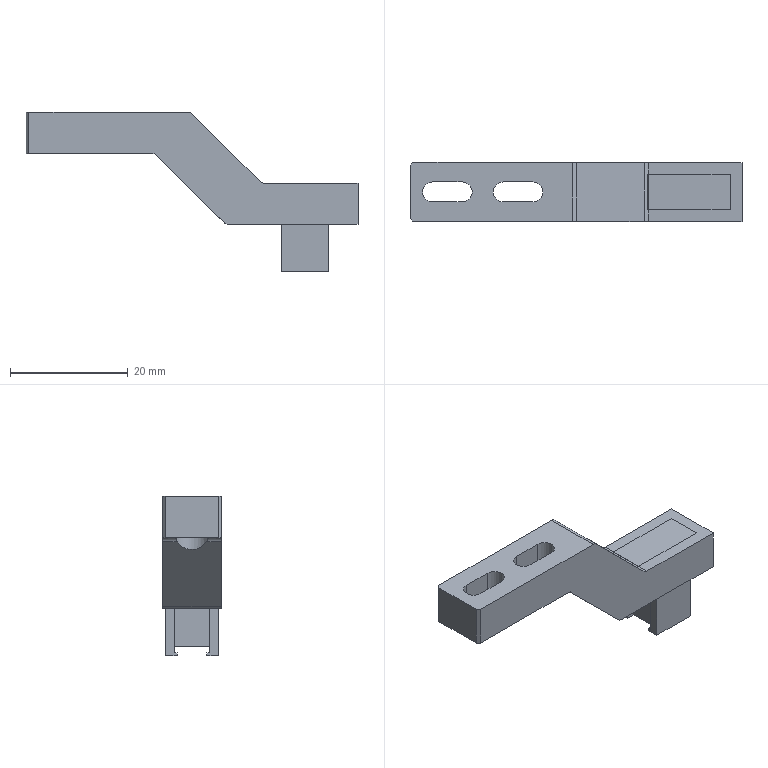NC program | NX | posted with a generic post | part box 56.3 x 10 x 27 mm
Lines 5635 to 5717 of 5717:
(ZLEVEL_PROFILE_1_COPY_1 , TOOL : D6A45)
N11220 T07 M6
N11222 G54
N11224 G17 G0 G90 X-19.32 Y0.741 S9500 M3
N11226 G43 Z30. H7
N11228 Z1.
N11230 G94 G1 Z-1. F1000.
N11232 X-24.32
N11234 G3 X-25.062 Y0. R0.741
N11236 X-24.32 Y-0.741 R0.741
N11238 G1 X-19.32
N11240 G3 X-18.579 Y0. R0.741
N11242 X-19.32 Y0.741 R0.741
N11244 X-19.84 Y0.441 R0.6
N11246 G1 Z0.
N11248 G0 Z30.
N11250 X-12.32 Y-0.741
N11252 Z1.
N11254 G1 Z-1.
N11256 X-7.32
N11258 G3 X-6.579 Y0. R0.741
N11260 X-7.32 Y0.741 R0.741
N11262 G1 X-12.32
N11264 G3 X-13.062 Y0. R0.741
N11266 X-12.32 Y-0.741 R0.741
N11268 X-11.801 Y-0.441 R0.6
N11270 G1 Z0.
N11272 G0 Z30.
N11274 X-0.361 Y-7.204
N11276 Z0.
N11278 G1 Z-1.
N11280 X-0.519 Y-6.41
N11282 G3 X-0.915 Y-5.959 R0.6
N11284 G1 X-27.651
N11286 G2 X-28.327 Y-5.678 R0.993
N11288 G1 X-28.828 Y-5.177
N11290 G2 X-29.109 Y-4.501 R0.957
N11292 G1 Y4.501
N11294 G2 X-28.828 Y5.177 R0.957
N11296 G1 X-28.327 Y5.678
N11298 G2 X-27.651 Y5.959 R0.993
N11300 G1 X-0.915
N11302 G3 X-0.519 Y6.41 R0.6
N11304 G1 X-0.361 Y7.204
N11306 Z0.
N11308 G0 Z30.
(ZLEVEL_PROFILE_1_COPY_1_COPY , TOOL : D6A45)
N11310 X14.648 Y-0.841
N11312 Z-12.
N11314 G1 Z-13.
N11316 X13.47 Y-1.522
N11318 G3 X13.17 Y-2.041 R0.6
N11320 G1 X25.191
N11322 Y2.041
N11324 X13.17
N11326 G3 X13.47 Y1.522 R0.6
N11328 G1 X14.648 Y0.841
N11330 Z-12.
N11332 G0 Z30.
N11334 X13.495 Y7.159
N11336 Z-12.
N11338 G1 Z-13.
N11340 X12.856 Y5.999
N11342 X12.9 Y5.967
N11344 X12.952 Y5.953
N11346 X13.006 Y5.959
N11348 X28.151
N11350 G2 X29.109 Y5.001 R0.958
N11352 G1 Y-5.001
N11354 G2 X28.151 Y-5.959 R0.958
N11356 G1 X13.007
N11358 X12.953 Y-5.953
N11360 X12.901 Y-5.967
N11362 X12.857 Y-5.999
N11364 X13.496 Y-7.159
N11366 Z-12.
N11368 G0 Z30.
N11370 M5
N11372 M2